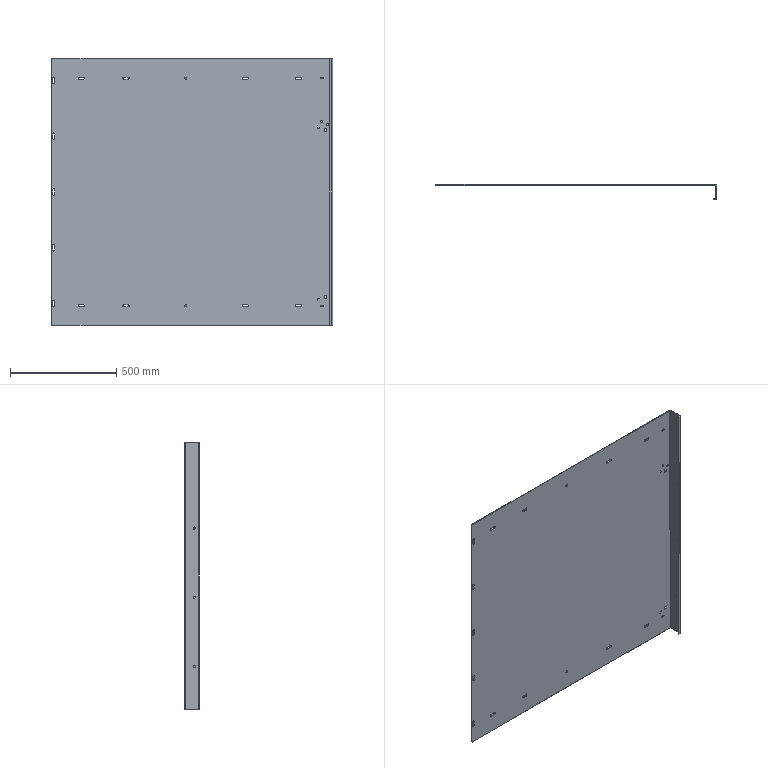Part | 1 solid | 123 faces | box 1320 x 70 x 1250 mm | volume 5226584 mm3 | plane 68 | cylinder 55 | commonest cylinder face diameters 10 x35 10.5 x10 8 x4 0.4 x2 4 x2 6.4 x2